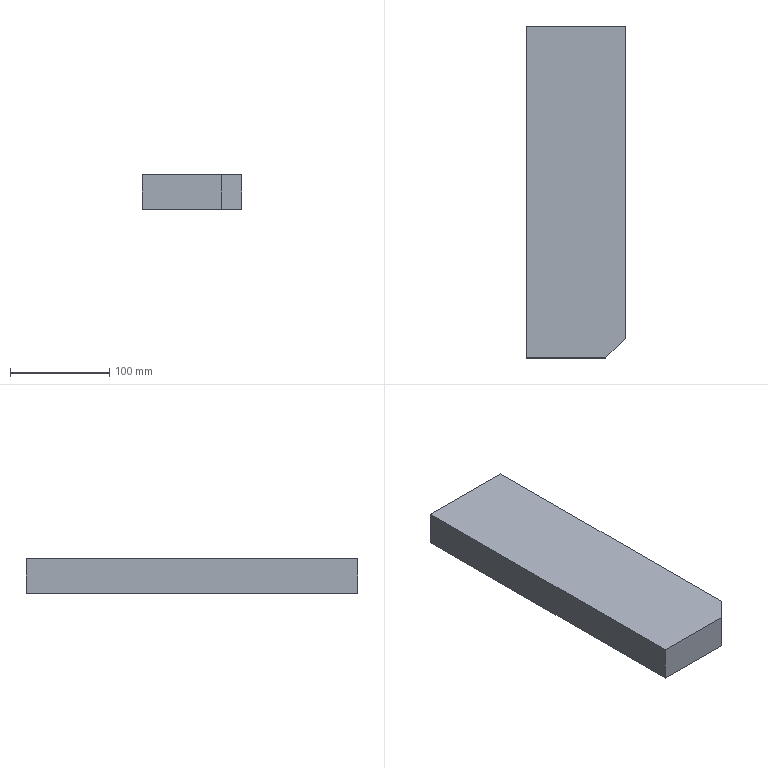Part | SolidWorks | features Chamfer 1, Extrusion 1 | 1 solid | 7 faces | box 100 x 335 x 35 mm | volume 1165500 mm3 | plane 7
STEP:
#1=CARTESIAN_POINT('',(0.,0.,0.));
#2=VERTEX_POINT('',#1);
#3=CARTESIAN_POINT('',(0.,-335.,0.));
#4=VERTEX_POINT('',#3);
#5=CARTESIAN_POINT('',(0.,0.,0.));
#6=DIRECTION('',(0.,-1.,0.));
#7=VECTOR('',#6,1000.);
#8=LINE('',#5,#7);
#9=EDGE_CURVE('',#2,#4,#8,.T.);
#10=ORIENTED_EDGE('',*,*,#9,.T.);
#11=CARTESIAN_POINT('',(0.,-335.,35.));
#12=VERTEX_POINT('',#11);
#13=CARTESIAN_POINT('',(0.,-335.,35.));
#14=DIRECTION('',(0.,0.,-1.));
#15=VECTOR('',#14,1000.);
#16=LINE('',#13,#15);
#17=EDGE_CURVE('',#12,#4,#16,.T.);
#18=ORIENTED_EDGE('',*,*,#17,.F.);
#19=CARTESIAN_POINT('',(0.,0.,35.));
#20=VERTEX_POINT('',#19);
#21=CARTESIAN_POINT('',(0.,0.,35.));
#22=DIRECTION('',(0.,-1.,0.));
#23=VECTOR('',#22,1000.);
#24=LINE('',#21,#23);
#25=EDGE_CURVE('',#20,#12,#24,.T.);
#26=ORIENTED_EDGE('',*,*,#25,.F.);
#27=CARTESIAN_POINT('',(0.,0.,35.));
#28=DIRECTION('',(0.,0.,-1.));
#29=VECTOR('',#28,1000.);
#30=LINE('',#27,#29);
#31=EDGE_CURVE('',#20,#2,#30,.T.);
#32=ORIENTED_EDGE('',*,*,#31,.T.);
#33=EDGE_LOOP('',(#10,#18,#26,#32));
#34=FACE_OUTER_BOUND('',#33,.T.);
#35=CARTESIAN_POINT('',(0.,0.,35.));
#36=DIRECTION('',(1.,0.,0.));
#37=DIRECTION('',(0.,0.,-1.));
#38=AXIS2_PLACEMENT_3D('',#35,#36,#37);
#39=PLANE('',#38);
#40=ADVANCED_FACE('',(#34),#39,.F.);
#41=CARTESIAN_POINT('',(80.,-335.,0.));
#42=VERTEX_POINT('',#41);
#43=CARTESIAN_POINT('',(0.,-335.,0.));
#44=DIRECTION('',(1.,0.,0.));
#45=VECTOR('',#44,1000.);
#46=LINE('',#43,#45);
#47=EDGE_CURVE('',#4,#42,#46,.T.);
#48=ORIENTED_EDGE('',*,*,#47,.T.);
#49=CARTESIAN_POINT('',(80.,-335.,35.));
#50=VERTEX_POINT('',#49);
#51=CARTESIAN_POINT('',(80.,-335.,35.));
#52=DIRECTION('',(0.,0.,1.));
#53=VECTOR('',#52,1000.);
#54=LINE('',#51,#53);
#55=EDGE_CURVE('',#42,#50,#54,.T.);
#56=ORIENTED_EDGE('',*,*,#55,.T.);
#57=CARTESIAN_POINT('',(0.,-335.,35.));
#58=DIRECTION('',(1.,0.,0.));
#59=VECTOR('',#58,1000.);
#60=LINE('',#57,#59);
#61=EDGE_CURVE('',#12,#50,#60,.T.);
#62=ORIENTED_EDGE('',*,*,#61,.F.);
#63=ORIENTED_EDGE('',*,*,#17,.T.);
#64=EDGE_LOOP('',(#48,#56,#62,#63));
#65=FACE_OUTER_BOUND('',#64,.T.);
#66=CARTESIAN_POINT('',(0.,-335.,35.));
#67=DIRECTION('',(0.,1.,0.));
#68=DIRECTION('',(0.,0.,1.));
#69=AXIS2_PLACEMENT_3D('',#66,#67,#68);
#70=PLANE('',#69);
#71=ADVANCED_FACE('',(#65),#70,.F.);
#72=CARTESIAN_POINT('',(100.,-315.,35.));
#73=VERTEX_POINT('',#72);
#74=CARTESIAN_POINT('',(100.,0.,35.));
#75=VERTEX_POINT('',#74);
#76=CARTESIAN_POINT('',(100.,0.,35.));
#77=DIRECTION('',(0.,1.,0.));
#78=VECTOR('',#77,1000.);
#79=LINE('',#76,#78);
#80=EDGE_CURVE('',#73,#75,#79,.T.);
#81=ORIENTED_EDGE('',*,*,#80,.F.);
#82=CARTESIAN_POINT('',(100.,-315.,0.));
#83=VERTEX_POINT('',#82);
#84=CARTESIAN_POINT('',(100.,-315.,35.));
#85=DIRECTION('',(0.,0.,-1.));
#86=VECTOR('',#85,1000.);
#87=LINE('',#84,#86);
#88=EDGE_CURVE('',#73,#83,#87,.T.);
#89=ORIENTED_EDGE('',*,*,#88,.T.);
#90=CARTESIAN_POINT('',(100.,0.,0.));
#91=VERTEX_POINT('',#90);
#92=CARTESIAN_POINT('',(100.,0.,0.));
#93=DIRECTION('',(0.,1.,0.));
#94=VECTOR('',#93,1000.);
#95=LINE('',#92,#94);
#96=EDGE_CURVE('',#83,#91,#95,.T.);
#97=ORIENTED_EDGE('',*,*,#96,.T.);
#98=CARTESIAN_POINT('',(100.,0.,35.));
#99=DIRECTION('',(0.,0.,-1.));
#100=VECTOR('',#99,1000.);
#101=LINE('',#98,#100);
#102=EDGE_CURVE('',#75,#91,#101,.T.);
#103=ORIENTED_EDGE('',*,*,#102,.F.);
#104=EDGE_LOOP('',(#81,#89,#97,#103));
#105=FACE_OUTER_BOUND('',#104,.T.);
#106=CARTESIAN_POINT('',(100.,0.,35.));
#107=DIRECTION('',(-1.,0.,0.));
#108=DIRECTION('',(0.,-1.,0.));
#109=AXIS2_PLACEMENT_3D('',#106,#107,#108);
#110=PLANE('',#109);
#111=ADVANCED_FACE('',(#105),#110,.F.);
#112=CARTESIAN_POINT('',(0.,0.,0.));
#113=DIRECTION('',(-1.,0.,0.));
#114=VECTOR('',#113,1000.);
#115=LINE('',#112,#114);
#116=EDGE_CURVE('',#91,#2,#115,.T.);
#117=ORIENTED_EDGE('',*,*,#116,.T.);
#118=ORIENTED_EDGE('',*,*,#31,.F.);
#119=CARTESIAN_POINT('',(0.,0.,35.));
#120=DIRECTION('',(-1.,0.,0.));
#121=VECTOR('',#120,1000.);
#122=LINE('',#119,#121);
#123=EDGE_CURVE('',#75,#20,#122,.T.);
#124=ORIENTED_EDGE('',*,*,#123,.F.);
#125=ORIENTED_EDGE('',*,*,#102,.T.);
#126=EDGE_LOOP('',(#117,#118,#124,#125));
#127=FACE_OUTER_BOUND('',#126,.T.);
#128=CARTESIAN_POINT('',(0.,0.,35.));
#129=DIRECTION('',(0.,-1.,0.));
#130=DIRECTION('',(0.,0.,-1.));
#131=AXIS2_PLACEMENT_3D('',#128,#129,#130);
#132=PLANE('',#131);
#133=ADVANCED_FACE('',(#127),#132,.F.);
#134=ORIENTED_EDGE('',*,*,#61,.T.);
#135=CARTESIAN_POINT('',(207.5,-207.5,35.));
#136=DIRECTION('',(0.7071,0.7071,0.));
#137=VECTOR('',#136,1000.);
#138=LINE('',#135,#137);
#139=EDGE_CURVE('',#50,#73,#138,.T.);
#140=ORIENTED_EDGE('',*,*,#139,.T.);
#141=ORIENTED_EDGE('',*,*,#80,.T.);
#142=ORIENTED_EDGE('',*,*,#123,.T.);
#143=ORIENTED_EDGE('',*,*,#25,.T.);
#144=EDGE_LOOP('',(#134,#140,#141,#142,#143));
#145=FACE_OUTER_BOUND('',#144,.T.);
#146=CARTESIAN_POINT('',(0.,0.,35.));
#147=DIRECTION('',(0.,0.,1.));
#148=DIRECTION('',(1.,0.,0.));
#149=AXIS2_PLACEMENT_3D('',#146,#147,#148);
#150=PLANE('',#149);
#151=ADVANCED_FACE('',(#145),#150,.T.);
#152=ORIENTED_EDGE('',*,*,#96,.F.);
#153=CARTESIAN_POINT('',(100.,-315.,0.));
#154=DIRECTION('',(-0.7071,-0.7071,0.));
#155=VECTOR('',#154,1000.);
#156=LINE('',#153,#155);
#157=EDGE_CURVE('',#83,#42,#156,.T.);
#158=ORIENTED_EDGE('',*,*,#157,.T.);
#159=ORIENTED_EDGE('',*,*,#47,.F.);
#160=ORIENTED_EDGE('',*,*,#9,.F.);
#161=ORIENTED_EDGE('',*,*,#116,.F.);
#162=EDGE_LOOP('',(#152,#158,#159,#160,#161));
#163=FACE_OUTER_BOUND('',#162,.T.);
#164=CARTESIAN_POINT('',(0.,0.,0.));
#165=DIRECTION('',(0.,0.,1.));
#166=DIRECTION('',(1.,0.,0.));
#167=AXIS2_PLACEMENT_3D('',#164,#165,#166);
#168=PLANE('',#167);
#169=ADVANCED_FACE('',(#163),#168,.F.);
#170=ORIENTED_EDGE('',*,*,#139,.F.);
#171=ORIENTED_EDGE('',*,*,#55,.F.);
#172=ORIENTED_EDGE('',*,*,#157,.F.);
#173=ORIENTED_EDGE('',*,*,#88,.F.);
#174=EDGE_LOOP('',(#170,#171,#172,#173));
#175=FACE_OUTER_BOUND('',#174,.T.);
#176=CARTESIAN_POINT('',(100.,-315.,35.));
#177=DIRECTION('',(-0.7071,0.7071,0.));
#178=DIRECTION('',(0.,0.,-1.));
#179=AXIS2_PLACEMENT_3D('',#176,#177,#178);
#180=PLANE('',#179);
#181=ADVANCED_FACE('',(#175),#180,.F.);
#182=CLOSED_SHELL('',(#40,#71,#111,#133,#151,#169,#181));
#183=MANIFOLD_SOLID_BREP('',#182);
#184=CARTESIAN_POINT('',(0.,0.,0.));
#185=DIRECTION('',(0.,0.,1.));
#186=DIRECTION('',(1.,0.,0.));
#187=AXIS2_PLACEMENT_3D('',#184,#185,#186);
#188=(LENGTH_UNIT()NAMED_UNIT(*)SI_UNIT(.MILLI.,.METRE.));
#189=UNCERTAINTY_MEASURE_WITH_UNIT(LENGTH_MEASURE(0.00001),#188,'','');
#190=(NAMED_UNIT(*)PLANE_ANGLE_UNIT()SI_UNIT($,.RADIAN.));
#191=(NAMED_UNIT(*)SI_UNIT($,.STERADIAN.)SOLID_ANGLE_UNIT());
#192=(GEOMETRIC_REPRESENTATION_CONTEXT(3)GLOBAL_UNCERTAINTY_ASSIGNED_CONTEXT((#189))GLOBAL_UNIT_ASSIGNED_CONTEXT((#188,#190,#191))REPRESENTATION_CONTEXT('',''));
#193=ADVANCED_BREP_SHAPE_REPRESENTATION('',(#183,#187),#192);